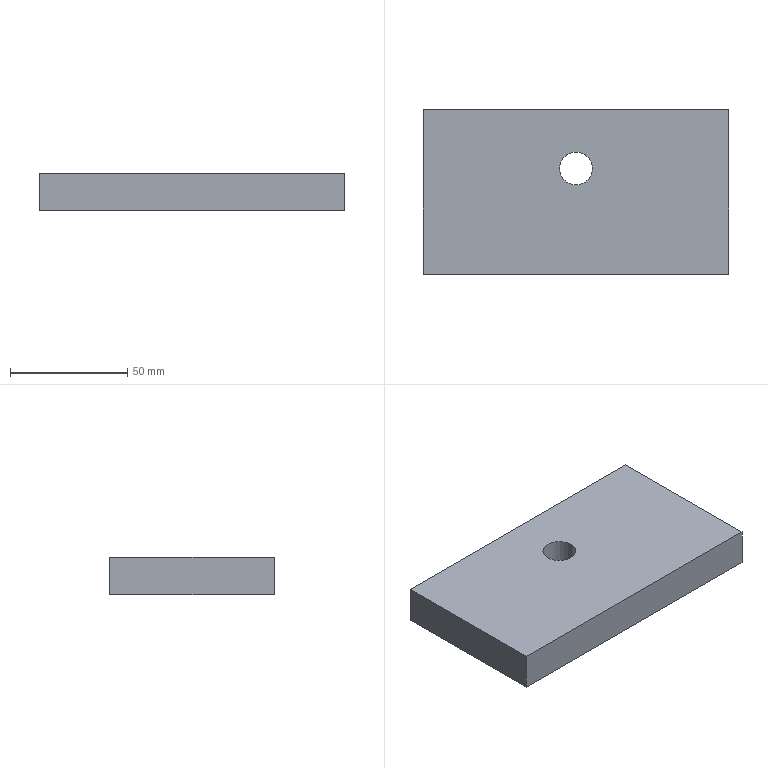Part | STEP file | 06-Base plate | 1 solid | 8 faces | box 130 x 70 x 16 mm | volume 143137 mm3 | plane 6 | cylinder 2 | commonest cylinder face diameters 14 x2
STEP:
#1=CARTESIAN_POINT('',(0.,0.,0.));
#2=DIRECTION('',(0.,0.,1.));
#3=DIRECTION('',(1.,0.,0.));
#4=AXIS2_PLACEMENT_3D('',#1,#2,#3);
#5=CARTESIAN_POINT('',(72.,-25.,0.));
#6=VERTEX_POINT('',#5);
#7=CARTESIAN_POINT('',(72.,-25.,16.));
#8=VERTEX_POINT('',#7);
#9=CARTESIAN_POINT('',(72.,-25.,16.));
#10=DIRECTION('',(0.,0.,1.));
#11=VECTOR('',#10,1.);
#12=LINE('',#9,#11);
#13=CARTESIAN_POINT('',(65.,-25.,16.));
#14=DIRECTION('',(0.,0.,1.));
#15=DIRECTION('',(1.,0.,0.));
#16=AXIS2_PLACEMENT_3D('',#13,#14,#15);
#17=CYLINDRICAL_SURFACE('',#16,7.);
#18=CARTESIAN_POINT('',(6.283,0.));
#19=DIRECTION('',(0.,1.));
#20=VECTOR('',#19,1.);
#21=LINE('',#18,#20);
#22=(GEOMETRIC_REPRESENTATION_CONTEXT(2)PARAMETRIC_REPRESENTATION_CONTEXT()REPRESENTATION_CONTEXT('',''));
#23=DEFINITIONAL_REPRESENTATION('',(#21),#22);
#24=PCURVE('',#17,#23);
#25=CARTESIAN_POINT('',(65.,-25.,16.));
#26=DIRECTION('',(0.,0.,1.));
#27=DIRECTION('',(1.,0.,0.));
#28=AXIS2_PLACEMENT_3D('',#25,#26,#27);
#29=CYLINDRICAL_SURFACE('',#28,7.);
#30=CARTESIAN_POINT('',(0.,0.));
#31=DIRECTION('',(0.,1.));
#32=VECTOR('',#31,1.);
#33=LINE('',#30,#32);
#34=(GEOMETRIC_REPRESENTATION_CONTEXT(2)PARAMETRIC_REPRESENTATION_CONTEXT()REPRESENTATION_CONTEXT('',''));
#35=DEFINITIONAL_REPRESENTATION('',(#33),#34);
#36=PCURVE('',#29,#35);
#37=SURFACE_CURVE('',#12,(#24,#36),.PCURVE_S1.);
#38=EDGE_CURVE('',#6,#8,#37,.T.);
#39=ORIENTED_EDGE('',*,*,#38,.T.);
#40=CARTESIAN_POINT('',(58.,-25.,16.));
#41=VERTEX_POINT('',#40);
#42=CARTESIAN_POINT('',(65.,-25.,16.));
#43=DIRECTION('',(0.,0.,1.));
#44=DIRECTION('',(1.,0.,0.));
#45=AXIS2_PLACEMENT_3D('',#42,#43,#44);
#46=CIRCLE('',#45,7.);
#47=CARTESIAN_POINT('',(0.,0.));
#48=DIRECTION('',(1.,0.));
#49=VECTOR('',#48,1.);
#50=LINE('',#47,#49);
#51=(GEOMETRIC_REPRESENTATION_CONTEXT(2)PARAMETRIC_REPRESENTATION_CONTEXT()REPRESENTATION_CONTEXT('',''));
#52=DEFINITIONAL_REPRESENTATION('',(#50),#51);
#53=PCURVE('',#17,#52);
#54=CARTESIAN_POINT('',(0.,0.,16.));
#55=DIRECTION('',(0.,0.,1.));
#56=DIRECTION('',(1.,0.,0.));
#57=AXIS2_PLACEMENT_3D('',#54,#55,#56);
#58=PLANE('',#57);
#59=CARTESIAN_POINT('',(65.,-25.));
#60=DIRECTION('',(1.,0.));
#61=AXIS2_PLACEMENT_2D('',#59,#60);
#62=CIRCLE('',#61,7.);
#63=(GEOMETRIC_REPRESENTATION_CONTEXT(2)PARAMETRIC_REPRESENTATION_CONTEXT()REPRESENTATION_CONTEXT('',''));
#64=DEFINITIONAL_REPRESENTATION('',(#62),#63);
#65=PCURVE('',#58,#64);
#66=SURFACE_CURVE('',#46,(#53,#65),.PCURVE_S1.);
#67=EDGE_CURVE('',#41,#8,#66,.T.);
#68=ORIENTED_EDGE('',*,*,#67,.F.);
#69=CARTESIAN_POINT('',(58.,-25.,0.));
#70=VERTEX_POINT('',#69);
#71=CARTESIAN_POINT('',(58.,-25.,16.));
#72=DIRECTION('',(0.,0.,1.));
#73=VECTOR('',#72,1.);
#74=LINE('',#71,#73);
#75=CARTESIAN_POINT('',(3.142,0.));
#76=DIRECTION('',(0.,1.));
#77=VECTOR('',#76,1.);
#78=LINE('',#75,#77);
#79=(GEOMETRIC_REPRESENTATION_CONTEXT(2)PARAMETRIC_REPRESENTATION_CONTEXT()REPRESENTATION_CONTEXT('',''));
#80=DEFINITIONAL_REPRESENTATION('',(#78),#79);
#81=PCURVE('',#17,#80);
#82=CARTESIAN_POINT('',(3.142,0.));
#83=DIRECTION('',(0.,1.));
#84=VECTOR('',#83,1.);
#85=LINE('',#82,#84);
#86=(GEOMETRIC_REPRESENTATION_CONTEXT(2)PARAMETRIC_REPRESENTATION_CONTEXT()REPRESENTATION_CONTEXT('',''));
#87=DEFINITIONAL_REPRESENTATION('',(#85),#86);
#88=PCURVE('',#29,#87);
#89=SURFACE_CURVE('',#74,(#81,#88),.PCURVE_S1.);
#90=EDGE_CURVE('',#70,#41,#89,.T.);
#91=ORIENTED_EDGE('',*,*,#90,.F.);
#92=CARTESIAN_POINT('',(65.,-25.,0.));
#93=DIRECTION('',(0.,0.,1.));
#94=DIRECTION('',(1.,0.,0.));
#95=AXIS2_PLACEMENT_3D('',#92,#93,#94);
#96=CIRCLE('',#95,7.);
#97=CARTESIAN_POINT('',(0.,-16.));
#98=DIRECTION('',(1.,0.));
#99=VECTOR('',#98,1.);
#100=LINE('',#97,#99);
#101=(GEOMETRIC_REPRESENTATION_CONTEXT(2)PARAMETRIC_REPRESENTATION_CONTEXT()REPRESENTATION_CONTEXT('',''));
#102=DEFINITIONAL_REPRESENTATION('',(#100),#101);
#103=PCURVE('',#17,#102);
#104=CARTESIAN_POINT('',(0.,0.,0.));
#105=DIRECTION('',(0.,0.,1.));
#106=DIRECTION('',(1.,0.,0.));
#107=AXIS2_PLACEMENT_3D('',#104,#105,#106);
#108=PLANE('',#107);
#109=CARTESIAN_POINT('',(65.,-25.));
#110=DIRECTION('',(1.,0.));
#111=AXIS2_PLACEMENT_2D('',#109,#110);
#112=CIRCLE('',#111,7.);
#113=(GEOMETRIC_REPRESENTATION_CONTEXT(2)PARAMETRIC_REPRESENTATION_CONTEXT()REPRESENTATION_CONTEXT('',''));
#114=DEFINITIONAL_REPRESENTATION('',(#112),#113);
#115=PCURVE('',#108,#114);
#116=SURFACE_CURVE('',#96,(#103,#115),.PCURVE_S1.);
#117=EDGE_CURVE('',#70,#6,#116,.T.);
#118=ORIENTED_EDGE('',*,*,#117,.T.);
#119=EDGE_LOOP('',(#39,#68,#91,#118));
#120=FACE_BOUND('',#119,.F.);
#121=ADVANCED_FACE('',(#120),#17,.F.);
#122=CARTESIAN_POINT('',(0.,0.,0.));
#123=VERTEX_POINT('',#122);
#124=CARTESIAN_POINT('',(0.,-70.,0.));
#125=VERTEX_POINT('',#124);
#126=CARTESIAN_POINT('',(0.,0.,0.));
#127=DIRECTION('',(0.,-1.,0.));
#128=VECTOR('',#127,1.);
#129=LINE('',#126,#128);
#130=CARTESIAN_POINT('',(0.,0.,16.));
#131=DIRECTION('',(1.,0.,0.));
#132=DIRECTION('',(0.,1.,0.));
#133=AXIS2_PLACEMENT_3D('',#130,#131,#132);
#134=PLANE('',#133);
#135=CARTESIAN_POINT('',(0.,-16.));
#136=DIRECTION('',(-1.,0.));
#137=VECTOR('',#136,1.);
#138=LINE('',#135,#137);
#139=(GEOMETRIC_REPRESENTATION_CONTEXT(2)PARAMETRIC_REPRESENTATION_CONTEXT()REPRESENTATION_CONTEXT('',''));
#140=DEFINITIONAL_REPRESENTATION('',(#138),#139);
#141=PCURVE('',#134,#140);
#142=CARTESIAN_POINT('',(0.,0.));
#143=DIRECTION('',(0.,-1.));
#144=VECTOR('',#143,1.);
#145=LINE('',#142,#144);
#146=(GEOMETRIC_REPRESENTATION_CONTEXT(2)PARAMETRIC_REPRESENTATION_CONTEXT()REPRESENTATION_CONTEXT('',''));
#147=DEFINITIONAL_REPRESENTATION('',(#145),#146);
#148=PCURVE('',#108,#147);
#149=SURFACE_CURVE('',#129,(#141,#148),.PCURVE_S1.);
#150=EDGE_CURVE('',#123,#125,#149,.T.);
#151=ORIENTED_EDGE('',*,*,#150,.T.);
#152=CARTESIAN_POINT('',(0.,-70.,16.));
#153=VERTEX_POINT('',#152);
#154=CARTESIAN_POINT('',(0.,-70.,16.));
#155=DIRECTION('',(0.,0.,-1.));
#156=VECTOR('',#155,1.);
#157=LINE('',#154,#156);
#158=CARTESIAN_POINT('',(-70.,0.));
#159=DIRECTION('',(0.,-1.));
#160=VECTOR('',#159,1.);
#161=LINE('',#158,#160);
#162=(GEOMETRIC_REPRESENTATION_CONTEXT(2)PARAMETRIC_REPRESENTATION_CONTEXT()REPRESENTATION_CONTEXT('',''));
#163=DEFINITIONAL_REPRESENTATION('',(#161),#162);
#164=PCURVE('',#134,#163);
#165=CARTESIAN_POINT('',(0.,-70.,16.));
#166=DIRECTION('',(0.,1.,0.));
#167=DIRECTION('',(0.,0.,1.));
#168=AXIS2_PLACEMENT_3D('',#165,#166,#167);
#169=PLANE('',#168);
#170=CARTESIAN_POINT('',(0.,0.));
#171=DIRECTION('',(-1.,0.));
#172=VECTOR('',#171,1.);
#173=LINE('',#170,#172);
#174=(GEOMETRIC_REPRESENTATION_CONTEXT(2)PARAMETRIC_REPRESENTATION_CONTEXT()REPRESENTATION_CONTEXT('',''));
#175=DEFINITIONAL_REPRESENTATION('',(#173),#174);
#176=PCURVE('',#169,#175);
#177=SURFACE_CURVE('',#157,(#164,#176),.PCURVE_S1.);
#178=EDGE_CURVE('',#153,#125,#177,.T.);
#179=ORIENTED_EDGE('',*,*,#178,.F.);
#180=CARTESIAN_POINT('',(0.,0.,16.));
#181=VERTEX_POINT('',#180);
#182=CARTESIAN_POINT('',(0.,0.,16.));
#183=DIRECTION('',(0.,-1.,0.));
#184=VECTOR('',#183,1.);
#185=LINE('',#182,#184);
#186=CARTESIAN_POINT('',(0.,0.));
#187=DIRECTION('',(-1.,0.));
#188=VECTOR('',#187,1.);
#189=LINE('',#186,#188);
#190=(GEOMETRIC_REPRESENTATION_CONTEXT(2)PARAMETRIC_REPRESENTATION_CONTEXT()REPRESENTATION_CONTEXT('',''));
#191=DEFINITIONAL_REPRESENTATION('',(#189),#190);
#192=PCURVE('',#134,#191);
#193=CARTESIAN_POINT('',(0.,0.));
#194=DIRECTION('',(0.,-1.));
#195=VECTOR('',#194,1.);
#196=LINE('',#193,#195);
#197=(GEOMETRIC_REPRESENTATION_CONTEXT(2)PARAMETRIC_REPRESENTATION_CONTEXT()REPRESENTATION_CONTEXT('',''));
#198=DEFINITIONAL_REPRESENTATION('',(#196),#197);
#199=PCURVE('',#58,#198);
#200=SURFACE_CURVE('',#185,(#192,#199),.PCURVE_S1.);
#201=EDGE_CURVE('',#181,#153,#200,.T.);
#202=ORIENTED_EDGE('',*,*,#201,.F.);
#203=CARTESIAN_POINT('',(0.,0.,16.));
#204=DIRECTION('',(0.,0.,-1.));
#205=VECTOR('',#204,1.);
#206=LINE('',#203,#205);
#207=CARTESIAN_POINT('',(0.,0.));
#208=DIRECTION('',(0.,-1.));
#209=VECTOR('',#208,1.);
#210=LINE('',#207,#209);
#211=(GEOMETRIC_REPRESENTATION_CONTEXT(2)PARAMETRIC_REPRESENTATION_CONTEXT()REPRESENTATION_CONTEXT('',''));
#212=DEFINITIONAL_REPRESENTATION('',(#210),#211);
#213=PCURVE('',#134,#212);
#214=CARTESIAN_POINT('',(0.,0.,16.));
#215=DIRECTION('',(0.,-1.,0.));
#216=DIRECTION('',(0.,0.,-1.));
#217=AXIS2_PLACEMENT_3D('',#214,#215,#216);
#218=PLANE('',#217);
#219=CARTESIAN_POINT('',(0.,0.));
#220=DIRECTION('',(1.,0.));
#221=VECTOR('',#220,1.);
#222=LINE('',#219,#221);
#223=(GEOMETRIC_REPRESENTATION_CONTEXT(2)PARAMETRIC_REPRESENTATION_CONTEXT()REPRESENTATION_CONTEXT('',''));
#224=DEFINITIONAL_REPRESENTATION('',(#222),#223);
#225=PCURVE('',#218,#224);
#226=SURFACE_CURVE('',#206,(#213,#225),.PCURVE_S1.);
#227=EDGE_CURVE('',#181,#123,#226,.T.);
#228=ORIENTED_EDGE('',*,*,#227,.T.);
#229=EDGE_LOOP('',(#151,#179,#202,#228));
#230=FACE_BOUND('',#229,.T.);
#231=ADVANCED_FACE('',(#230),#134,.F.);
#232=CARTESIAN_POINT('',(130.,-70.,0.));
#233=VERTEX_POINT('',#232);
#234=CARTESIAN_POINT('',(0.,-70.,0.));
#235=DIRECTION('',(1.,0.,0.));
#236=VECTOR('',#235,1.);
#237=LINE('',#234,#236);
#238=CARTESIAN_POINT('',(-16.,0.));
#239=DIRECTION('',(0.,1.));
#240=VECTOR('',#239,1.);
#241=LINE('',#238,#240);
#242=(GEOMETRIC_REPRESENTATION_CONTEXT(2)PARAMETRIC_REPRESENTATION_CONTEXT()REPRESENTATION_CONTEXT('',''));
#243=DEFINITIONAL_REPRESENTATION('',(#241),#242);
#244=PCURVE('',#169,#243);
#245=CARTESIAN_POINT('',(0.,-70.));
#246=DIRECTION('',(1.,0.));
#247=VECTOR('',#246,1.);
#248=LINE('',#245,#247);
#249=(GEOMETRIC_REPRESENTATION_CONTEXT(2)PARAMETRIC_REPRESENTATION_CONTEXT()REPRESENTATION_CONTEXT('',''));
#250=DEFINITIONAL_REPRESENTATION('',(#248),#249);
#251=PCURVE('',#108,#250);
#252=SURFACE_CURVE('',#237,(#244,#251),.PCURVE_S1.);
#253=EDGE_CURVE('',#125,#233,#252,.T.);
#254=ORIENTED_EDGE('',*,*,#253,.T.);
#255=CARTESIAN_POINT('',(130.,-70.,16.));
#256=VERTEX_POINT('',#255);
#257=CARTESIAN_POINT('',(130.,-70.,16.));
#258=DIRECTION('',(0.,0.,-1.));
#259=VECTOR('',#258,1.);
#260=LINE('',#257,#259);
#261=CARTESIAN_POINT('',(0.,130.));
#262=DIRECTION('',(-1.,0.));
#263=VECTOR('',#262,1.);
#264=LINE('',#261,#263);
#265=(GEOMETRIC_REPRESENTATION_CONTEXT(2)PARAMETRIC_REPRESENTATION_CONTEXT()REPRESENTATION_CONTEXT('',''));
#266=DEFINITIONAL_REPRESENTATION('',(#264),#265);
#267=PCURVE('',#169,#266);
#268=CARTESIAN_POINT('',(130.,0.,16.));
#269=DIRECTION('',(-1.,0.,0.));
#270=DIRECTION('',(0.,0.,1.));
#271=AXIS2_PLACEMENT_3D('',#268,#269,#270);
#272=PLANE('',#271);
#273=CARTESIAN_POINT('',(0.,-70.));
#274=DIRECTION('',(-1.,0.));
#275=VECTOR('',#274,1.);
#276=LINE('',#273,#275);
#277=(GEOMETRIC_REPRESENTATION_CONTEXT(2)PARAMETRIC_REPRESENTATION_CONTEXT()REPRESENTATION_CONTEXT('',''));
#278=DEFINITIONAL_REPRESENTATION('',(#276),#277);
#279=PCURVE('',#272,#278);
#280=SURFACE_CURVE('',#260,(#267,#279),.PCURVE_S1.);
#281=EDGE_CURVE('',#256,#233,#280,.T.);
#282=ORIENTED_EDGE('',*,*,#281,.F.);
#283=CARTESIAN_POINT('',(0.,-70.,16.));
#284=DIRECTION('',(1.,0.,0.));
#285=VECTOR('',#284,1.);
#286=LINE('',#283,#285);
#287=CARTESIAN_POINT('',(0.,0.));
#288=DIRECTION('',(0.,1.));
#289=VECTOR('',#288,1.);
#290=LINE('',#287,#289);
#291=(GEOMETRIC_REPRESENTATION_CONTEXT(2)PARAMETRIC_REPRESENTATION_CONTEXT()REPRESENTATION_CONTEXT('',''));
#292=DEFINITIONAL_REPRESENTATION('',(#290),#291);
#293=PCURVE('',#169,#292);
#294=CARTESIAN_POINT('',(0.,-70.));
#295=DIRECTION('',(1.,0.));
#296=VECTOR('',#295,1.);
#297=LINE('',#294,#296);
#298=(GEOMETRIC_REPRESENTATION_CONTEXT(2)PARAMETRIC_REPRESENTATION_CONTEXT()REPRESENTATION_CONTEXT('',''));
#299=DEFINITIONAL_REPRESENTATION('',(#297),#298);
#300=PCURVE('',#58,#299);
#301=SURFACE_CURVE('',#286,(#293,#300),.PCURVE_S1.);
#302=EDGE_CURVE('',#153,#256,#301,.T.);
#303=ORIENTED_EDGE('',*,*,#302,.F.);
#304=ORIENTED_EDGE('',*,*,#178,.T.);
#305=EDGE_LOOP('',(#254,#282,#303,#304));
#306=FACE_BOUND('',#305,.T.);
#307=ADVANCED_FACE('',(#306),#169,.F.);
#308=CARTESIAN_POINT('',(130.,0.,0.));
#309=VERTEX_POINT('',#308);
#310=CARTESIAN_POINT('',(130.,0.,0.));
#311=DIRECTION('',(0.,1.,0.));
#312=VECTOR('',#311,1.);
#313=LINE('',#310,#312);
#314=CARTESIAN_POINT('',(-16.,0.));
#315=DIRECTION('',(0.,1.));
#316=VECTOR('',#315,1.);
#317=LINE('',#314,#316);
#318=(GEOMETRIC_REPRESENTATION_CONTEXT(2)PARAMETRIC_REPRESENTATION_CONTEXT()REPRESENTATION_CONTEXT('',''));
#319=DEFINITIONAL_REPRESENTATION('',(#317),#318);
#320=PCURVE('',#272,#319);
#321=CARTESIAN_POINT('',(130.,0.));
#322=DIRECTION('',(0.,1.));
#323=VECTOR('',#322,1.);
#324=LINE('',#321,#323);
#325=(GEOMETRIC_REPRESENTATION_CONTEXT(2)PARAMETRIC_REPRESENTATION_CONTEXT()REPRESENTATION_CONTEXT('',''));
#326=DEFINITIONAL_REPRESENTATION('',(#324),#325);
#327=PCURVE('',#108,#326);
#328=SURFACE_CURVE('',#313,(#320,#327),.PCURVE_S1.);
#329=EDGE_CURVE('',#233,#309,#328,.T.);
#330=ORIENTED_EDGE('',*,*,#329,.T.);
#331=CARTESIAN_POINT('',(130.,0.,16.));
#332=VERTEX_POINT('',#331);
#333=CARTESIAN_POINT('',(130.,0.,16.));
#334=DIRECTION('',(0.,0.,-1.));
#335=VECTOR('',#334,1.);
#336=LINE('',#333,#335);
#337=CARTESIAN_POINT('',(0.,0.));
#338=DIRECTION('',(-1.,0.));
#339=VECTOR('',#338,1.);
#340=LINE('',#337,#339);
#341=(GEOMETRIC_REPRESENTATION_CONTEXT(2)PARAMETRIC_REPRESENTATION_CONTEXT()REPRESENTATION_CONTEXT('',''));
#342=DEFINITIONAL_REPRESENTATION('',(#340),#341);
#343=PCURVE('',#272,#342);
#344=CARTESIAN_POINT('',(0.,130.));
#345=DIRECTION('',(1.,0.));
#346=VECTOR('',#345,1.);
#347=LINE('',#344,#346);
#348=(GEOMETRIC_REPRESENTATION_CONTEXT(2)PARAMETRIC_REPRESENTATION_CONTEXT()REPRESENTATION_CONTEXT('',''));
#349=DEFINITIONAL_REPRESENTATION('',(#347),#348);
#350=PCURVE('',#218,#349);
#351=SURFACE_CURVE('',#336,(#343,#350),.PCURVE_S1.);
#352=EDGE_CURVE('',#332,#309,#351,.T.);
#353=ORIENTED_EDGE('',*,*,#352,.F.);
#354=CARTESIAN_POINT('',(130.,0.,16.));
#355=DIRECTION('',(0.,1.,0.));
#356=VECTOR('',#355,1.);
#357=LINE('',#354,#356);
#358=CARTESIAN_POINT('',(0.,0.));
#359=DIRECTION('',(0.,1.));
#360=VECTOR('',#359,1.);
#361=LINE('',#358,#360);
#362=(GEOMETRIC_REPRESENTATION_CONTEXT(2)PARAMETRIC_REPRESENTATION_CONTEXT()REPRESENTATION_CONTEXT('',''));
#363=DEFINITIONAL_REPRESENTATION('',(#361),#362);
#364=PCURVE('',#272,#363);
#365=CARTESIAN_POINT('',(130.,0.));
#366=DIRECTION('',(0.,1.));
#367=VECTOR('',#366,1.);
#368=LINE('',#365,#367);
#369=(GEOMETRIC_REPRESENTATION_CONTEXT(2)PARAMETRIC_REPRESENTATION_CONTEXT()REPRESENTATION_CONTEXT('',''));
#370=DEFINITIONAL_REPRESENTATION('',(#368),#369);
#371=PCURVE('',#58,#370);
#372=SURFACE_CURVE('',#357,(#364,#371),.PCURVE_S1.);
#373=EDGE_CURVE('',#256,#332,#372,.T.);
#374=ORIENTED_EDGE('',*,*,#373,.F.);
#375=ORIENTED_EDGE('',*,*,#281,.T.);
#376=EDGE_LOOP('',(#330,#353,#374,#375));
#377=FACE_BOUND('',#376,.T.);
#378=ADVANCED_FACE('',(#377),#272,.F.);
#379=CARTESIAN_POINT('',(0.,0.,0.));
#380=DIRECTION('',(-1.,0.,0.));
#381=VECTOR('',#380,1.);
#382=LINE('',#379,#381);
#383=CARTESIAN_POINT('',(16.,0.));
#384=DIRECTION('',(0.,-1.));
#385=VECTOR('',#384,1.);
#386=LINE('',#383,#385);
#387=(GEOMETRIC_REPRESENTATION_CONTEXT(2)PARAMETRIC_REPRESENTATION_CONTEXT()REPRESENTATION_CONTEXT('',''));
#388=DEFINITIONAL_REPRESENTATION('',(#386),#387);
#389=PCURVE('',#218,#388);
#390=CARTESIAN_POINT('',(0.,0.));
#391=DIRECTION('',(-1.,0.));
#392=VECTOR('',#391,1.);
#393=LINE('',#390,#392);
#394=(GEOMETRIC_REPRESENTATION_CONTEXT(2)PARAMETRIC_REPRESENTATION_CONTEXT()REPRESENTATION_CONTEXT('',''));
#395=DEFINITIONAL_REPRESENTATION('',(#393),#394);
#396=PCURVE('',#108,#395);
#397=SURFACE_CURVE('',#382,(#389,#396),.PCURVE_S1.);
#398=EDGE_CURVE('',#309,#123,#397,.T.);
#399=ORIENTED_EDGE('',*,*,#398,.T.);
#400=ORIENTED_EDGE('',*,*,#227,.F.);
#401=CARTESIAN_POINT('',(0.,0.,16.));
#402=DIRECTION('',(-1.,0.,0.));
#403=VECTOR('',#402,1.);
#404=LINE('',#401,#403);
#405=CARTESIAN_POINT('',(0.,0.));
#406=DIRECTION('',(0.,-1.));
#407=VECTOR('',#406,1.);
#408=LINE('',#405,#407);
#409=(GEOMETRIC_REPRESENTATION_CONTEXT(2)PARAMETRIC_REPRESENTATION_CONTEXT()REPRESENTATION_CONTEXT('',''));
#410=DEFINITIONAL_REPRESENTATION('',(#408),#409);
#411=PCURVE('',#218,#410);
#412=CARTESIAN_POINT('',(0.,0.));
#413=DIRECTION('',(-1.,0.));
#414=VECTOR('',#413,1.);
#415=LINE('',#412,#414);
#416=(GEOMETRIC_REPRESENTATION_CONTEXT(2)PARAMETRIC_REPRESENTATION_CONTEXT()REPRESENTATION_CONTEXT('',''));
#417=DEFINITIONAL_REPRESENTATION('',(#415),#416);
#418=PCURVE('',#58,#417);
#419=SURFACE_CURVE('',#404,(#411,#418),.PCURVE_S1.);
#420=EDGE_CURVE('',#332,#181,#419,.T.);
#421=ORIENTED_EDGE('',*,*,#420,.F.);
#422=ORIENTED_EDGE('',*,*,#352,.T.);
#423=EDGE_LOOP('',(#399,#400,#421,#422));
#424=FACE_BOUND('',#423,.T.);
#425=ADVANCED_FACE('',(#424),#218,.F.);
#426=CARTESIAN_POINT('',(65.,-25.,16.));
#427=DIRECTION('',(0.,0.,1.));
#428=DIRECTION('',(1.,0.,0.));
#429=AXIS2_PLACEMENT_3D('',#426,#427,#428);
#430=CIRCLE('',#429,7.);
#431=CARTESIAN_POINT('',(65.,-25.));
#432=DIRECTION('',(1.,0.));
#433=AXIS2_PLACEMENT_2D('',#431,#432);
#434=CIRCLE('',#433,7.);
#435=(GEOMETRIC_REPRESENTATION_CONTEXT(2)PARAMETRIC_REPRESENTATION_CONTEXT()REPRESENTATION_CONTEXT('',''));
#436=DEFINITIONAL_REPRESENTATION('',(#434),#435);
#437=PCURVE('',#58,#436);
#438=CARTESIAN_POINT('',(0.,0.));
#439=DIRECTION('',(1.,0.));
#440=VECTOR('',#439,1.);
#441=LINE('',#438,#440);
#442=(GEOMETRIC_REPRESENTATION_CONTEXT(2)PARAMETRIC_REPRESENTATION_CONTEXT()REPRESENTATION_CONTEXT('',''));
#443=DEFINITIONAL_REPRESENTATION('',(#441),#442);
#444=PCURVE('',#29,#443);
#445=SURFACE_CURVE('',#430,(#437,#444),.PCURVE_S1.);
#446=EDGE_CURVE('',#8,#41,#445,.T.);
#447=ORIENTED_EDGE('',*,*,#446,.F.);
#448=ORIENTED_EDGE('',*,*,#67,.F.);
#449=EDGE_LOOP('',(#447,#448));
#450=FACE_BOUND('',#449,.T.);
#451=ORIENTED_EDGE('',*,*,#201,.T.);
#452=ORIENTED_EDGE('',*,*,#302,.T.);
#453=ORIENTED_EDGE('',*,*,#373,.T.);
#454=ORIENTED_EDGE('',*,*,#420,.T.);
#455=EDGE_LOOP('',(#451,#452,#453,#454));
#456=FACE_BOUND('',#455,.T.);
#457=ADVANCED_FACE('',(#450,#456),#58,.T.);
#458=CARTESIAN_POINT('',(65.,-25.,0.));
#459=DIRECTION('',(0.,0.,1.));
#460=DIRECTION('',(1.,0.,0.));
#461=AXIS2_PLACEMENT_3D('',#458,#459,#460);
#462=CIRCLE('',#461,7.);
#463=CARTESIAN_POINT('',(65.,-25.));
#464=DIRECTION('',(1.,0.));
#465=AXIS2_PLACEMENT_2D('',#463,#464);
#466=CIRCLE('',#465,7.);
#467=(GEOMETRIC_REPRESENTATION_CONTEXT(2)PARAMETRIC_REPRESENTATION_CONTEXT()REPRESENTATION_CONTEXT('',''));
#468=DEFINITIONAL_REPRESENTATION('',(#466),#467);
#469=PCURVE('',#108,#468);
#470=CARTESIAN_POINT('',(0.,-16.));
#471=DIRECTION('',(1.,0.));
#472=VECTOR('',#471,1.);
#473=LINE('',#470,#472);
#474=(GEOMETRIC_REPRESENTATION_CONTEXT(2)PARAMETRIC_REPRESENTATION_CONTEXT()REPRESENTATION_CONTEXT('',''));
#475=DEFINITIONAL_REPRESENTATION('',(#473),#474);
#476=PCURVE('',#29,#475);
#477=SURFACE_CURVE('',#462,(#469,#476),.PCURVE_S1.);
#478=EDGE_CURVE('',#6,#70,#477,.T.);
#479=ORIENTED_EDGE('',*,*,#478,.T.);
#480=ORIENTED_EDGE('',*,*,#117,.T.);
#481=EDGE_LOOP('',(#479,#480));
#482=FACE_BOUND('',#481,.T.);
#483=ORIENTED_EDGE('',*,*,#150,.F.);
#484=ORIENTED_EDGE('',*,*,#398,.F.);
#485=ORIENTED_EDGE('',*,*,#329,.F.);
#486=ORIENTED_EDGE('',*,*,#253,.F.);
#487=EDGE_LOOP('',(#483,#484,#485,#486));
#488=FACE_BOUND('',#487,.T.);
#489=ADVANCED_FACE('',(#482,#488),#108,.F.);
#490=ORIENTED_EDGE('',*,*,#446,.F.);
#491=ORIENTED_EDGE('',*,*,#38,.F.);
#492=ORIENTED_EDGE('',*,*,#478,.T.);
#493=ORIENTED_EDGE('',*,*,#90,.T.);
#494=EDGE_LOOP('',(#490,#491,#492,#493));
#495=FACE_BOUND('',#494,.F.);
#496=ADVANCED_FACE('',(#495),#29,.F.);
#497=CLOSED_SHELL('',(#121,#231,#307,#378,#425,#457,#489,#496));
#498=MANIFOLD_SOLID_BREP('',#497);
#499=(LENGTH_UNIT()NAMED_UNIT(*)SI_UNIT(.MILLI.,.METRE.));
#500=UNCERTAINTY_MEASURE_WITH_UNIT(LENGTH_MEASURE(0.0000001),#499,'','');
#501=(NAMED_UNIT(*)PLANE_ANGLE_UNIT()SI_UNIT($,.RADIAN.));
#502=(NAMED_UNIT(*)SI_UNIT($,.STERADIAN.)SOLID_ANGLE_UNIT());
#503=(GEOMETRIC_REPRESENTATION_CONTEXT(3)GLOBAL_UNCERTAINTY_ASSIGNED_CONTEXT((#500))GLOBAL_UNIT_ASSIGNED_CONTEXT((#499,#501,#502))REPRESENTATION_CONTEXT('',''));
#504=ADVANCED_BREP_SHAPE_REPRESENTATION('',(#4,#498),#503);